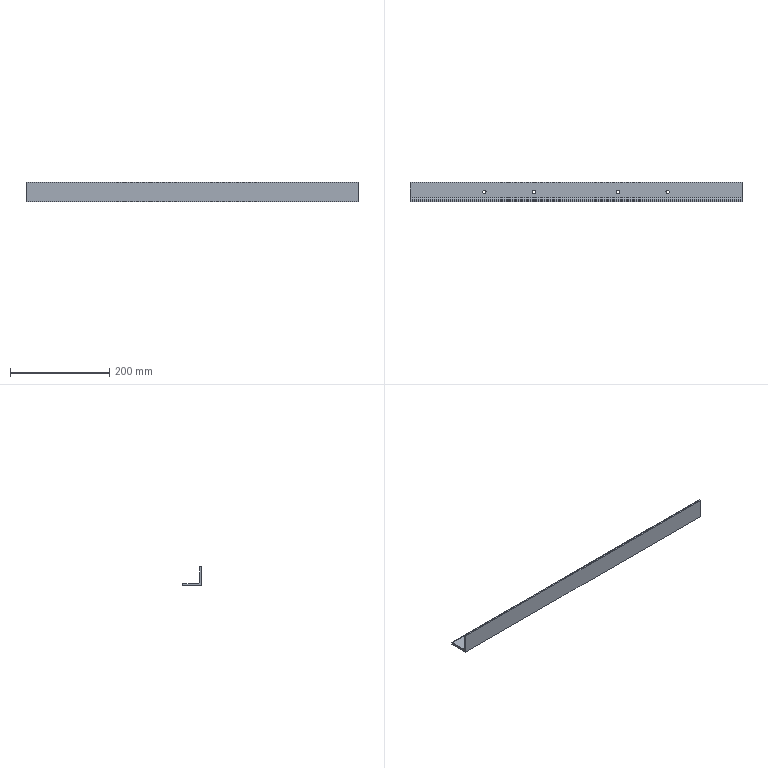Part | SolidWorks | features BaseBody 1 | 1 solid | 19 faces | box 670 x 40 x 40 mm | volume 206182 mm3 | cylinder 11 | plane 8 | commonest cylinder face diameters 6.8 x8 2.667 x2 10 x1
STEP:
#1=CARTESIAN_POINT('',(188.4,20.,4.));
#2=VERTEX_POINT('',#1);
#3=CARTESIAN_POINT('',(181.6,20.,4.));
#4=VERTEX_POINT('',#3);
#5=CARTESIAN_POINT('',(185.,20.,4.));
#6=DIRECTION('',(0.,0.,-1.));
#7=DIRECTION('',(0.,1.,0.));
#8=AXIS2_PLACEMENT_3D('',#5,#6,#7);
#9=CIRCLE('',#8,3.4);
#10=EDGE_CURVE('',#2,#4,#9,.T.);
#11=ORIENTED_EDGE('',*,*,#10,.F.);
#12=CARTESIAN_POINT('',(188.4,20.,0.));
#13=VERTEX_POINT('',#12);
#14=CARTESIAN_POINT('',(188.4,20.,0.));
#15=DIRECTION('',(0.,0.,-1.));
#16=VECTOR('',#15,1000.);
#17=LINE('',#14,#16);
#18=EDGE_CURVE('',#2,#13,#17,.T.);
#19=ORIENTED_EDGE('',*,*,#18,.T.);
#20=CARTESIAN_POINT('',(181.6,20.,0.));
#21=VERTEX_POINT('',#20);
#22=CARTESIAN_POINT('',(185.,20.,0.));
#23=DIRECTION('',(0.,0.,-1.));
#24=DIRECTION('',(-1.,0.,0.));
#25=AXIS2_PLACEMENT_3D('',#22,#23,#24);
#26=CIRCLE('',#25,3.4);
#27=EDGE_CURVE('',#13,#21,#26,.T.);
#28=ORIENTED_EDGE('',*,*,#27,.T.);
#29=CARTESIAN_POINT('',(181.6,20.,0.));
#30=DIRECTION('',(0.,0.,-1.));
#31=VECTOR('',#30,1000.);
#32=LINE('',#29,#31);
#33=EDGE_CURVE('',#4,#21,#32,.T.);
#34=ORIENTED_EDGE('',*,*,#33,.F.);
#35=EDGE_LOOP('',(#11,#19,#28,#34));
#36=FACE_OUTER_BOUND('',#35,.T.);
#37=CARTESIAN_POINT('',(185.,20.,0.));
#38=DIRECTION('',(0.,0.,-1.));
#39=DIRECTION('',(-1.,0.,0.));
#40=AXIS2_PLACEMENT_3D('',#37,#38,#39);
#41=CYLINDRICAL_SURFACE('',#40,3.4);
#42=ADVANCED_FACE('',(#36),#41,.F.);
#43=CARTESIAN_POINT('',(88.4,20.,4.));
#44=VERTEX_POINT('',#43);
#45=CARTESIAN_POINT('',(81.6,20.,4.));
#46=VERTEX_POINT('',#45);
#47=CARTESIAN_POINT('',(85.,20.,4.));
#48=DIRECTION('',(0.,0.,-1.));
#49=DIRECTION('',(0.,1.,0.));
#50=AXIS2_PLACEMENT_3D('',#47,#48,#49);
#51=CIRCLE('',#50,3.4);
#52=EDGE_CURVE('',#44,#46,#51,.T.);
#53=ORIENTED_EDGE('',*,*,#52,.F.);
#54=CARTESIAN_POINT('',(88.4,20.,0.));
#55=VERTEX_POINT('',#54);
#56=CARTESIAN_POINT('',(88.4,20.,0.));
#57=DIRECTION('',(0.,0.,-1.));
#58=VECTOR('',#57,1000.);
#59=LINE('',#56,#58);
#60=EDGE_CURVE('',#44,#55,#59,.T.);
#61=ORIENTED_EDGE('',*,*,#60,.T.);
#62=CARTESIAN_POINT('',(81.6,20.,0.));
#63=VERTEX_POINT('',#62);
#64=CARTESIAN_POINT('',(85.,20.,0.));
#65=DIRECTION('',(0.,0.,-1.));
#66=DIRECTION('',(-1.,0.,0.));
#67=AXIS2_PLACEMENT_3D('',#64,#65,#66);
#68=CIRCLE('',#67,3.4);
#69=EDGE_CURVE('',#55,#63,#68,.T.);
#70=ORIENTED_EDGE('',*,*,#69,.T.);
#71=CARTESIAN_POINT('',(81.6,20.,0.));
#72=DIRECTION('',(0.,0.,-1.));
#73=VECTOR('',#72,1000.);
#74=LINE('',#71,#73);
#75=EDGE_CURVE('',#46,#63,#74,.T.);
#76=ORIENTED_EDGE('',*,*,#75,.F.);
#77=EDGE_LOOP('',(#53,#61,#70,#76));
#78=FACE_OUTER_BOUND('',#77,.T.);
#79=CARTESIAN_POINT('',(85.,20.,0.));
#80=DIRECTION('',(0.,0.,-1.));
#81=DIRECTION('',(-1.,0.,0.));
#82=AXIS2_PLACEMENT_3D('',#79,#80,#81);
#83=CYLINDRICAL_SURFACE('',#82,3.4);
#84=ADVANCED_FACE('',(#78),#83,.F.);
#85=CARTESIAN_POINT('',(-181.6,20.,4.));
#86=VERTEX_POINT('',#85);
#87=CARTESIAN_POINT('',(-188.4,20.,4.));
#88=VERTEX_POINT('',#87);
#89=CARTESIAN_POINT('',(-185.,20.,4.));
#90=DIRECTION('',(0.,0.,-1.));
#91=DIRECTION('',(0.,1.,0.));
#92=AXIS2_PLACEMENT_3D('',#89,#90,#91);
#93=CIRCLE('',#92,3.4);
#94=EDGE_CURVE('',#86,#88,#93,.T.);
#95=ORIENTED_EDGE('',*,*,#94,.F.);
#96=CARTESIAN_POINT('',(-181.6,20.,0.));
#97=VERTEX_POINT('',#96);
#98=CARTESIAN_POINT('',(-181.6,20.,0.));
#99=DIRECTION('',(0.,0.,-1.));
#100=VECTOR('',#99,1000.);
#101=LINE('',#98,#100);
#102=EDGE_CURVE('',#86,#97,#101,.T.);
#103=ORIENTED_EDGE('',*,*,#102,.T.);
#104=CARTESIAN_POINT('',(-188.4,20.,0.));
#105=VERTEX_POINT('',#104);
#106=CARTESIAN_POINT('',(-185.,20.,0.));
#107=DIRECTION('',(0.,0.,-1.));
#108=DIRECTION('',(-1.,0.,0.));
#109=AXIS2_PLACEMENT_3D('',#106,#107,#108);
#110=CIRCLE('',#109,3.4);
#111=EDGE_CURVE('',#97,#105,#110,.T.);
#112=ORIENTED_EDGE('',*,*,#111,.T.);
#113=CARTESIAN_POINT('',(-188.4,20.,0.));
#114=DIRECTION('',(0.,0.,-1.));
#115=VECTOR('',#114,1000.);
#116=LINE('',#113,#115);
#117=EDGE_CURVE('',#88,#105,#116,.T.);
#118=ORIENTED_EDGE('',*,*,#117,.F.);
#119=EDGE_LOOP('',(#95,#103,#112,#118));
#120=FACE_OUTER_BOUND('',#119,.T.);
#121=CARTESIAN_POINT('',(-185.,20.,0.));
#122=DIRECTION('',(0.,0.,-1.));
#123=DIRECTION('',(-1.,0.,0.));
#124=AXIS2_PLACEMENT_3D('',#121,#122,#123);
#125=CYLINDRICAL_SURFACE('',#124,3.4);
#126=ADVANCED_FACE('',(#120),#125,.F.);
#127=CARTESIAN_POINT('',(-81.6,20.,4.));
#128=VERTEX_POINT('',#127);
#129=CARTESIAN_POINT('',(-88.4,20.,4.));
#130=VERTEX_POINT('',#129);
#131=CARTESIAN_POINT('',(-85.,20.,4.));
#132=DIRECTION('',(0.,0.,-1.));
#133=DIRECTION('',(0.,1.,0.));
#134=AXIS2_PLACEMENT_3D('',#131,#132,#133);
#135=CIRCLE('',#134,3.4);
#136=EDGE_CURVE('',#128,#130,#135,.T.);
#137=ORIENTED_EDGE('',*,*,#136,.F.);
#138=CARTESIAN_POINT('',(-81.6,20.,0.));
#139=VERTEX_POINT('',#138);
#140=CARTESIAN_POINT('',(-81.6,20.,0.));
#141=DIRECTION('',(0.,0.,-1.));
#142=VECTOR('',#141,1000.);
#143=LINE('',#140,#142);
#144=EDGE_CURVE('',#128,#139,#143,.T.);
#145=ORIENTED_EDGE('',*,*,#144,.T.);
#146=CARTESIAN_POINT('',(-88.4,20.,0.));
#147=VERTEX_POINT('',#146);
#148=CARTESIAN_POINT('',(-85.,20.,0.));
#149=DIRECTION('',(0.,0.,-1.));
#150=DIRECTION('',(-1.,0.,0.));
#151=AXIS2_PLACEMENT_3D('',#148,#149,#150);
#152=CIRCLE('',#151,3.4);
#153=EDGE_CURVE('',#139,#147,#152,.T.);
#154=ORIENTED_EDGE('',*,*,#153,.T.);
#155=CARTESIAN_POINT('',(-88.4,20.,0.));
#156=DIRECTION('',(0.,0.,-1.));
#157=VECTOR('',#156,1000.);
#158=LINE('',#155,#157);
#159=EDGE_CURVE('',#130,#147,#158,.T.);
#160=ORIENTED_EDGE('',*,*,#159,.F.);
#161=EDGE_LOOP('',(#137,#145,#154,#160));
#162=FACE_OUTER_BOUND('',#161,.T.);
#163=CARTESIAN_POINT('',(-85.,20.,0.));
#164=DIRECTION('',(0.,0.,-1.));
#165=DIRECTION('',(-1.,0.,0.));
#166=AXIS2_PLACEMENT_3D('',#163,#164,#165);
#167=CYLINDRICAL_SURFACE('',#166,3.4);
#168=ADVANCED_FACE('',(#162),#167,.F.);
#169=CARTESIAN_POINT('',(185.,20.,0.));
#170=DIRECTION('',(0.,0.,-1.));
#171=DIRECTION('',(-1.,0.,0.));
#172=AXIS2_PLACEMENT_3D('',#169,#170,#171);
#173=CIRCLE('',#172,3.4);
#174=EDGE_CURVE('',#21,#13,#173,.T.);
#175=ORIENTED_EDGE('',*,*,#174,.F.);
#176=ORIENTED_EDGE('',*,*,#27,.F.);
#177=EDGE_LOOP('',(#175,#176));
#178=FACE_BOUND('',#177,.T.);
#179=CARTESIAN_POINT('',(85.,20.,0.));
#180=DIRECTION('',(0.,0.,-1.));
#181=DIRECTION('',(-1.,0.,0.));
#182=AXIS2_PLACEMENT_3D('',#179,#180,#181);
#183=CIRCLE('',#182,3.4);
#184=EDGE_CURVE('',#63,#55,#183,.T.);
#185=ORIENTED_EDGE('',*,*,#184,.F.);
#186=ORIENTED_EDGE('',*,*,#69,.F.);
#187=EDGE_LOOP('',(#185,#186));
#188=FACE_BOUND('',#187,.T.);
#189=CARTESIAN_POINT('',(-185.,20.,0.));
#190=DIRECTION('',(0.,0.,-1.));
#191=DIRECTION('',(-1.,0.,0.));
#192=AXIS2_PLACEMENT_3D('',#189,#190,#191);
#193=CIRCLE('',#192,3.4);
#194=EDGE_CURVE('',#105,#97,#193,.T.);
#195=ORIENTED_EDGE('',*,*,#194,.F.);
#196=ORIENTED_EDGE('',*,*,#111,.F.);
#197=EDGE_LOOP('',(#195,#196));
#198=FACE_BOUND('',#197,.T.);
#199=CARTESIAN_POINT('',(-85.,20.,0.));
#200=DIRECTION('',(0.,0.,-1.));
#201=DIRECTION('',(-1.,0.,0.));
#202=AXIS2_PLACEMENT_3D('',#199,#200,#201);
#203=CIRCLE('',#202,3.4);
#204=EDGE_CURVE('',#147,#139,#203,.T.);
#205=ORIENTED_EDGE('',*,*,#204,.F.);
#206=ORIENTED_EDGE('',*,*,#153,.F.);
#207=EDGE_LOOP('',(#205,#206));
#208=FACE_BOUND('',#207,.T.);
#209=CARTESIAN_POINT('',(-335.,0.,0.));
#210=VERTEX_POINT('',#209);
#211=CARTESIAN_POINT('',(-335.,40.,0.));
#212=VERTEX_POINT('',#211);
#213=CARTESIAN_POINT('',(-335.,40.,0.));
#214=DIRECTION('',(0.,1.,0.));
#215=VECTOR('',#214,1000.);
#216=LINE('',#213,#215);
#217=EDGE_CURVE('',#210,#212,#216,.T.);
#218=ORIENTED_EDGE('',*,*,#217,.T.);
#219=CARTESIAN_POINT('',(335.,40.,0.));
#220=VERTEX_POINT('',#219);
#221=CARTESIAN_POINT('',(335.,40.,0.));
#222=DIRECTION('',(-1.,0.,0.));
#223=VECTOR('',#222,1000.);
#224=LINE('',#221,#223);
#225=EDGE_CURVE('',#220,#212,#224,.T.);
#226=ORIENTED_EDGE('',*,*,#225,.F.);
#227=CARTESIAN_POINT('',(335.,0.,0.));
#228=VERTEX_POINT('',#227);
#229=CARTESIAN_POINT('',(335.,40.,0.));
#230=DIRECTION('',(0.,1.,0.));
#231=VECTOR('',#230,1000.);
#232=LINE('',#229,#231);
#233=EDGE_CURVE('',#228,#220,#232,.T.);
#234=ORIENTED_EDGE('',*,*,#233,.F.);
#235=CARTESIAN_POINT('',(335.,0.,0.));
#236=DIRECTION('',(-1.,0.,0.));
#237=VECTOR('',#236,1000.);
#238=LINE('',#235,#237);
#239=EDGE_CURVE('',#228,#210,#238,.T.);
#240=ORIENTED_EDGE('',*,*,#239,.T.);
#241=EDGE_LOOP('',(#218,#226,#234,#240));
#242=FACE_OUTER_BOUND('',#241,.T.);
#243=CARTESIAN_POINT('',(335.,40.,0.));
#244=DIRECTION('',(0.,0.,1.));
#245=DIRECTION('',(1.,0.,0.));
#246=AXIS2_PLACEMENT_3D('',#243,#244,#245);
#247=PLANE('',#246);
#248=ADVANCED_FACE('',(#178,#188,#198,#208,#242),#247,.F.);
#249=CARTESIAN_POINT('',(-335.,40.,2.667));
#250=VERTEX_POINT('',#249);
#251=CARTESIAN_POINT('',(-335.,40.,0.));
#252=DIRECTION('',(0.,0.,1.));
#253=VECTOR('',#252,1000.);
#254=LINE('',#251,#253);
#255=EDGE_CURVE('',#212,#250,#254,.T.);
#256=ORIENTED_EDGE('',*,*,#255,.T.);
#257=CARTESIAN_POINT('',(335.,40.,2.667));
#258=VERTEX_POINT('',#257);
#259=CARTESIAN_POINT('',(335.,40.,2.667));
#260=DIRECTION('',(-1.,0.,0.));
#261=VECTOR('',#260,1000.);
#262=LINE('',#259,#261);
#263=EDGE_CURVE('',#258,#250,#262,.T.);
#264=ORIENTED_EDGE('',*,*,#263,.F.);
#265=CARTESIAN_POINT('',(335.,40.,0.));
#266=DIRECTION('',(0.,0.,1.));
#267=VECTOR('',#266,1000.);
#268=LINE('',#265,#267);
#269=EDGE_CURVE('',#220,#258,#268,.T.);
#270=ORIENTED_EDGE('',*,*,#269,.F.);
#271=ORIENTED_EDGE('',*,*,#225,.T.);
#272=EDGE_LOOP('',(#256,#264,#270,#271));
#273=FACE_OUTER_BOUND('',#272,.T.);
#274=CARTESIAN_POINT('',(335.,40.,0.));
#275=DIRECTION('',(0.,-1.,0.));
#276=DIRECTION('',(0.,0.,-1.));
#277=AXIS2_PLACEMENT_3D('',#274,#275,#276);
#278=PLANE('',#277);
#279=ADVANCED_FACE('',(#273),#278,.F.);
#280=CARTESIAN_POINT('',(-335.,38.667,4.));
#281=VERTEX_POINT('',#280);
#282=CARTESIAN_POINT('',(-335.,38.667,2.667));
#283=DIRECTION('',(1.,0.,0.));
#284=DIRECTION('',(0.,0.,-1.));
#285=AXIS2_PLACEMENT_3D('',#282,#283,#284);
#286=CIRCLE('',#285,1.333);
#287=EDGE_CURVE('',#250,#281,#286,.T.);
#288=ORIENTED_EDGE('',*,*,#287,.T.);
#289=CARTESIAN_POINT('',(335.,38.667,4.));
#290=VERTEX_POINT('',#289);
#291=CARTESIAN_POINT('',(335.,38.667,4.));
#292=DIRECTION('',(-1.,0.,0.));
#293=VECTOR('',#292,1000.);
#294=LINE('',#291,#293);
#295=EDGE_CURVE('',#290,#281,#294,.T.);
#296=ORIENTED_EDGE('',*,*,#295,.F.);
#297=CARTESIAN_POINT('',(335.,38.667,2.667));
#298=DIRECTION('',(1.,0.,0.));
#299=DIRECTION('',(0.,0.,-1.));
#300=AXIS2_PLACEMENT_3D('',#297,#298,#299);
#301=CIRCLE('',#300,1.333);
#302=EDGE_CURVE('',#258,#290,#301,.T.);
#303=ORIENTED_EDGE('',*,*,#302,.F.);
#304=ORIENTED_EDGE('',*,*,#263,.T.);
#305=EDGE_LOOP('',(#288,#296,#303,#304));
#306=FACE_OUTER_BOUND('',#305,.T.);
#307=CARTESIAN_POINT('',(335.,38.667,2.667));
#308=DIRECTION('',(-1.,0.,0.));
#309=DIRECTION('',(0.,0.,1.));
#310=AXIS2_PLACEMENT_3D('',#307,#308,#309);
#311=CYLINDRICAL_SURFACE('',#310,1.333);
#312=ADVANCED_FACE('',(#306),#311,.T.);
#313=CARTESIAN_POINT('',(185.,20.,4.));
#314=DIRECTION('',(0.,0.,-1.));
#315=DIRECTION('',(0.,1.,0.));
#316=AXIS2_PLACEMENT_3D('',#313,#314,#315);
#317=CIRCLE('',#316,3.4);
#318=EDGE_CURVE('',#4,#2,#317,.T.);
#319=ORIENTED_EDGE('',*,*,#318,.T.);
#320=ORIENTED_EDGE('',*,*,#10,.T.);
#321=EDGE_LOOP('',(#319,#320));
#322=FACE_BOUND('',#321,.T.);
#323=CARTESIAN_POINT('',(85.,20.,4.));
#324=DIRECTION('',(0.,0.,-1.));
#325=DIRECTION('',(0.,1.,0.));
#326=AXIS2_PLACEMENT_3D('',#323,#324,#325);
#327=CIRCLE('',#326,3.4);
#328=EDGE_CURVE('',#46,#44,#327,.T.);
#329=ORIENTED_EDGE('',*,*,#328,.T.);
#330=ORIENTED_EDGE('',*,*,#52,.T.);
#331=EDGE_LOOP('',(#329,#330));
#332=FACE_BOUND('',#331,.T.);
#333=CARTESIAN_POINT('',(-185.,20.,4.));
#334=DIRECTION('',(0.,0.,-1.));
#335=DIRECTION('',(0.,1.,0.));
#336=AXIS2_PLACEMENT_3D('',#333,#334,#335);
#337=CIRCLE('',#336,3.4);
#338=EDGE_CURVE('',#88,#86,#337,.T.);
#339=ORIENTED_EDGE('',*,*,#338,.T.);
#340=ORIENTED_EDGE('',*,*,#94,.T.);
#341=EDGE_LOOP('',(#339,#340));
#342=FACE_BOUND('',#341,.T.);
#343=CARTESIAN_POINT('',(-85.,20.,4.));
#344=DIRECTION('',(0.,0.,-1.));
#345=DIRECTION('',(0.,1.,0.));
#346=AXIS2_PLACEMENT_3D('',#343,#344,#345);
#347=CIRCLE('',#346,3.4);
#348=EDGE_CURVE('',#130,#128,#347,.T.);
#349=ORIENTED_EDGE('',*,*,#348,.T.);
#350=ORIENTED_EDGE('',*,*,#136,.T.);
#351=EDGE_LOOP('',(#349,#350));
#352=FACE_BOUND('',#351,.T.);
#353=CARTESIAN_POINT('',(-335.,9.,4.));
#354=VERTEX_POINT('',#353);
#355=CARTESIAN_POINT('',(-335.,9.,4.));
#356=DIRECTION('',(0.,-1.,0.));
#357=VECTOR('',#356,1000.);
#358=LINE('',#355,#357);
#359=EDGE_CURVE('',#281,#354,#358,.T.);
#360=ORIENTED_EDGE('',*,*,#359,.T.);
#361=CARTESIAN_POINT('',(335.,9.,4.));
#362=VERTEX_POINT('',#361);
#363=CARTESIAN_POINT('',(335.,9.,4.));
#364=DIRECTION('',(-1.,0.,0.));
#365=VECTOR('',#364,1000.);
#366=LINE('',#363,#365);
#367=EDGE_CURVE('',#362,#354,#366,.T.);
#368=ORIENTED_EDGE('',*,*,#367,.F.);
#369=CARTESIAN_POINT('',(335.,9.,4.));
#370=DIRECTION('',(0.,-1.,0.));
#371=VECTOR('',#370,1000.);
#372=LINE('',#369,#371);
#373=EDGE_CURVE('',#290,#362,#372,.T.);
#374=ORIENTED_EDGE('',*,*,#373,.F.);
#375=ORIENTED_EDGE('',*,*,#295,.T.);
#376=EDGE_LOOP('',(#360,#368,#374,#375));
#377=FACE_OUTER_BOUND('',#376,.T.);
#378=CARTESIAN_POINT('',(335.,9.,4.));
#379=DIRECTION('',(0.,0.,-1.));
#380=DIRECTION('',(0.,1.,0.));
#381=AXIS2_PLACEMENT_3D('',#378,#379,#380);
#382=PLANE('',#381);
#383=ADVANCED_FACE('',(#322,#332,#342,#352,#377),#382,.F.);
#384=CARTESIAN_POINT('',(-335.,4.,9.));
#385=VERTEX_POINT('',#384);
#386=CARTESIAN_POINT('',(-335.,9.,9.));
#387=DIRECTION('',(-1.,0.,0.));
#388=DIRECTION('',(0.,0.,1.));
#389=AXIS2_PLACEMENT_3D('',#386,#387,#388);
#390=CIRCLE('',#389,5.);
#391=EDGE_CURVE('',#354,#385,#390,.T.);
#392=ORIENTED_EDGE('',*,*,#391,.T.);
#393=CARTESIAN_POINT('',(335.,4.,9.));
#394=VERTEX_POINT('',#393);
#395=CARTESIAN_POINT('',(335.,4.,9.));
#396=DIRECTION('',(-1.,0.,0.));
#397=VECTOR('',#396,1000.);
#398=LINE('',#395,#397);
#399=EDGE_CURVE('',#394,#385,#398,.T.);
#400=ORIENTED_EDGE('',*,*,#399,.F.);
#401=CARTESIAN_POINT('',(335.,9.,9.));
#402=DIRECTION('',(-1.,0.,0.));
#403=DIRECTION('',(0.,0.,1.));
#404=AXIS2_PLACEMENT_3D('',#401,#402,#403);
#405=CIRCLE('',#404,5.);
#406=EDGE_CURVE('',#362,#394,#405,.T.);
#407=ORIENTED_EDGE('',*,*,#406,.F.);
#408=ORIENTED_EDGE('',*,*,#367,.T.);
#409=EDGE_LOOP('',(#392,#400,#407,#408));
#410=FACE_OUTER_BOUND('',#409,.T.);
#411=CARTESIAN_POINT('',(335.,9.,9.));
#412=DIRECTION('',(-1.,0.,0.));
#413=DIRECTION('',(0.,0.,1.));
#414=AXIS2_PLACEMENT_3D('',#411,#412,#413);
#415=CYLINDRICAL_SURFACE('',#414,5.);
#416=ADVANCED_FACE('',(#410),#415,.F.);
#417=CARTESIAN_POINT('',(-335.,4.,38.667));
#418=VERTEX_POINT('',#417);
#419=CARTESIAN_POINT('',(-335.,4.,38.667));
#420=DIRECTION('',(0.,0.,1.));
#421=VECTOR('',#420,1000.);
#422=LINE('',#419,#421);
#423=EDGE_CURVE('',#385,#418,#422,.T.);
#424=ORIENTED_EDGE('',*,*,#423,.T.);
#425=CARTESIAN_POINT('',(335.,4.,38.667));
#426=VERTEX_POINT('',#425);
#427=CARTESIAN_POINT('',(335.,4.,38.667));
#428=DIRECTION('',(-1.,0.,0.));
#429=VECTOR('',#428,1000.);
#430=LINE('',#427,#429);
#431=EDGE_CURVE('',#426,#418,#430,.T.);
#432=ORIENTED_EDGE('',*,*,#431,.F.);
#433=CARTESIAN_POINT('',(335.,4.,38.667));
#434=DIRECTION('',(0.,0.,1.));
#435=VECTOR('',#434,1000.);
#436=LINE('',#433,#435);
#437=EDGE_CURVE('',#394,#426,#436,.T.);
#438=ORIENTED_EDGE('',*,*,#437,.F.);
#439=ORIENTED_EDGE('',*,*,#399,.T.);
#440=EDGE_LOOP('',(#424,#432,#438,#439));
#441=FACE_OUTER_BOUND('',#440,.T.);
#442=CARTESIAN_POINT('',(335.,4.,38.667));
#443=DIRECTION('',(0.,-1.,0.));
#444=DIRECTION('',(0.,0.,-1.));
#445=AXIS2_PLACEMENT_3D('',#442,#443,#444);
#446=PLANE('',#445);
#447=ADVANCED_FACE('',(#441),#446,.F.);
#448=CARTESIAN_POINT('',(-335.,2.667,40.));
#449=VERTEX_POINT('',#448);
#450=CARTESIAN_POINT('',(-335.,2.667,38.667));
#451=DIRECTION('',(1.,0.,0.));
#452=DIRECTION('',(0.,0.,1.));
#453=AXIS2_PLACEMENT_3D('',#450,#451,#452);
#454=CIRCLE('',#453,1.333);
#455=EDGE_CURVE('',#418,#449,#454,.T.);
#456=ORIENTED_EDGE('',*,*,#455,.T.);
#457=CARTESIAN_POINT('',(335.,2.667,40.));
#458=VERTEX_POINT('',#457);
#459=CARTESIAN_POINT('',(335.,2.667,40.));
#460=DIRECTION('',(-1.,0.,0.));
#461=VECTOR('',#460,1000.);
#462=LINE('',#459,#461);
#463=EDGE_CURVE('',#458,#449,#462,.T.);
#464=ORIENTED_EDGE('',*,*,#463,.F.);
#465=CARTESIAN_POINT('',(335.,2.667,38.667));
#466=DIRECTION('',(1.,0.,0.));
#467=DIRECTION('',(0.,0.,1.));
#468=AXIS2_PLACEMENT_3D('',#465,#466,#467);
#469=CIRCLE('',#468,1.333);
#470=EDGE_CURVE('',#426,#458,#469,.T.);
#471=ORIENTED_EDGE('',*,*,#470,.F.);
#472=ORIENTED_EDGE('',*,*,#431,.T.);
#473=EDGE_LOOP('',(#456,#464,#471,#472));
#474=FACE_OUTER_BOUND('',#473,.T.);
#475=CARTESIAN_POINT('',(335.,2.667,38.667));
#476=DIRECTION('',(-1.,0.,0.));
#477=DIRECTION('',(0.,0.,1.));
#478=AXIS2_PLACEMENT_3D('',#475,#476,#477);
#479=CYLINDRICAL_SURFACE('',#478,1.333);
#480=ADVANCED_FACE('',(#474),#479,.T.);
#481=CARTESIAN_POINT('',(-335.,0.,40.));
#482=VERTEX_POINT('',#481);
#483=CARTESIAN_POINT('',(-335.,0.,40.));
#484=DIRECTION('',(0.,-1.,0.));
#485=VECTOR('',#484,1000.);
#486=LINE('',#483,#485);
#487=EDGE_CURVE('',#449,#482,#486,.T.);
#488=ORIENTED_EDGE('',*,*,#487,.T.);
#489=CARTESIAN_POINT('',(335.,0.,40.));
#490=VERTEX_POINT('',#489);
#491=CARTESIAN_POINT('',(335.,0.,40.));
#492=DIRECTION('',(-1.,0.,0.));
#493=VECTOR('',#492,1000.);
#494=LINE('',#491,#493);
#495=EDGE_CURVE('',#490,#482,#494,.T.);
#496=ORIENTED_EDGE('',*,*,#495,.F.);
#497=CARTESIAN_POINT('',(335.,0.,40.));
#498=DIRECTION('',(0.,-1.,0.));
#499=VECTOR('',#498,1000.);
#500=LINE('',#497,#499);
#501=EDGE_CURVE('',#458,#490,#500,.T.);
#502=ORIENTED_EDGE('',*,*,#501,.F.);
#503=ORIENTED_EDGE('',*,*,#463,.T.);
#504=EDGE_LOOP('',(#488,#496,#502,#503));
#505=FACE_OUTER_BOUND('',#504,.T.);
#506=CARTESIAN_POINT('',(335.,0.,40.));
#507=DIRECTION('',(0.,0.,-1.));
#508=DIRECTION('',(-1.,0.,0.));
#509=AXIS2_PLACEMENT_3D('',#506,#507,#508);
#510=PLANE('',#509);
#511=ADVANCED_FACE('',(#505),#510,.F.);
#512=CARTESIAN_POINT('',(-335.,0.,0.));
#513=DIRECTION('',(0.,0.,-1.));
#514=VECTOR('',#513,1000.);
#515=LINE('',#512,#514);
#516=EDGE_CURVE('',#482,#210,#515,.T.);
#517=ORIENTED_EDGE('',*,*,#516,.T.);
#518=ORIENTED_EDGE('',*,*,#239,.F.);
#519=CARTESIAN_POINT('',(335.,0.,0.));
#520=DIRECTION('',(0.,0.,-1.));
#521=VECTOR('',#520,1000.);
#522=LINE('',#519,#521);
#523=EDGE_CURVE('',#490,#228,#522,.T.);
#524=ORIENTED_EDGE('',*,*,#523,.F.);
#525=ORIENTED_EDGE('',*,*,#495,.T.);
#526=EDGE_LOOP('',(#517,#518,#524,#525));
#527=FACE_OUTER_BOUND('',#526,.T.);
#528=CARTESIAN_POINT('',(335.,0.,0.));
#529=DIRECTION('',(0.,1.,0.));
#530=DIRECTION('',(0.,0.,1.));
#531=AXIS2_PLACEMENT_3D('',#528,#529,#530);
#532=PLANE('',#531);
#533=ADVANCED_FACE('',(#527),#532,.F.);
#534=ORIENTED_EDGE('',*,*,#233,.T.);
#535=ORIENTED_EDGE('',*,*,#269,.T.);
#536=ORIENTED_EDGE('',*,*,#302,.T.);
#537=ORIENTED_EDGE('',*,*,#373,.T.);
#538=ORIENTED_EDGE('',*,*,#406,.T.);
#539=ORIENTED_EDGE('',*,*,#437,.T.);
#540=ORIENTED_EDGE('',*,*,#470,.T.);
#541=ORIENTED_EDGE('',*,*,#501,.T.);
#542=ORIENTED_EDGE('',*,*,#523,.T.);
#543=EDGE_LOOP('',(#534,#535,#536,#537,#538,#539,#540,#541,#542));
#544=FACE_OUTER_BOUND('',#543,.T.);
#545=CARTESIAN_POINT('',(335.,2.667,38.667));
#546=DIRECTION('',(-1.,0.,0.));
#547=DIRECTION('',(0.,0.,1.));
#548=AXIS2_PLACEMENT_3D('',#545,#546,#547);
#549=PLANE('',#548);
#550=ADVANCED_FACE('',(#544),#549,.F.);
#551=ORIENTED_EDGE('',*,*,#217,.F.);
#552=ORIENTED_EDGE('',*,*,#516,.F.);
#553=ORIENTED_EDGE('',*,*,#487,.F.);
#554=ORIENTED_EDGE('',*,*,#455,.F.);
#555=ORIENTED_EDGE('',*,*,#423,.F.);
#556=ORIENTED_EDGE('',*,*,#391,.F.);
#557=ORIENTED_EDGE('',*,*,#359,.F.);
#558=ORIENTED_EDGE('',*,*,#287,.F.);
#559=ORIENTED_EDGE('',*,*,#255,.F.);
#560=EDGE_LOOP('',(#551,#552,#553,#554,#555,#556,#557,#558,#559));
#561=FACE_OUTER_BOUND('',#560,.T.);
#562=CARTESIAN_POINT('',(-335.,2.667,38.667));
#563=DIRECTION('',(-1.,0.,0.));
#564=DIRECTION('',(0.,0.,1.));
#565=AXIS2_PLACEMENT_3D('',#562,#563,#564);
#566=PLANE('',#565);
#567=ADVANCED_FACE('',(#561),#566,.T.);
#568=ORIENTED_EDGE('',*,*,#144,.F.);
#569=ORIENTED_EDGE('',*,*,#348,.F.);
#570=ORIENTED_EDGE('',*,*,#159,.T.);
#571=ORIENTED_EDGE('',*,*,#204,.T.);
#572=EDGE_LOOP('',(#568,#569,#570,#571));
#573=FACE_OUTER_BOUND('',#572,.T.);
#574=CARTESIAN_POINT('',(-85.,20.,0.));
#575=DIRECTION('',(0.,0.,-1.));
#576=DIRECTION('',(-1.,0.,0.));
#577=AXIS2_PLACEMENT_3D('',#574,#575,#576);
#578=CYLINDRICAL_SURFACE('',#577,3.4);
#579=ADVANCED_FACE('',(#573),#578,.F.);
#580=ORIENTED_EDGE('',*,*,#102,.F.);
#581=ORIENTED_EDGE('',*,*,#338,.F.);
#582=ORIENTED_EDGE('',*,*,#117,.T.);
#583=ORIENTED_EDGE('',*,*,#194,.T.);
#584=EDGE_LOOP('',(#580,#581,#582,#583));
#585=FACE_OUTER_BOUND('',#584,.T.);
#586=CARTESIAN_POINT('',(-185.,20.,0.));
#587=DIRECTION('',(0.,0.,-1.));
#588=DIRECTION('',(-1.,0.,0.));
#589=AXIS2_PLACEMENT_3D('',#586,#587,#588);
#590=CYLINDRICAL_SURFACE('',#589,3.4);
#591=ADVANCED_FACE('',(#585),#590,.F.);
#592=ORIENTED_EDGE('',*,*,#60,.F.);
#593=ORIENTED_EDGE('',*,*,#328,.F.);
#594=ORIENTED_EDGE('',*,*,#75,.T.);
#595=ORIENTED_EDGE('',*,*,#184,.T.);
#596=EDGE_LOOP('',(#592,#593,#594,#595));
#597=FACE_OUTER_BOUND('',#596,.T.);
#598=CARTESIAN_POINT('',(85.,20.,0.));
#599=DIRECTION('',(0.,0.,-1.));
#600=DIRECTION('',(-1.,0.,0.));
#601=AXIS2_PLACEMENT_3D('',#598,#599,#600);
#602=CYLINDRICAL_SURFACE('',#601,3.4);
#603=ADVANCED_FACE('',(#597),#602,.F.);
#604=ORIENTED_EDGE('',*,*,#18,.F.);
#605=ORIENTED_EDGE('',*,*,#318,.F.);
#606=ORIENTED_EDGE('',*,*,#33,.T.);
#607=ORIENTED_EDGE('',*,*,#174,.T.);
#608=EDGE_LOOP('',(#604,#605,#606,#607));
#609=FACE_OUTER_BOUND('',#608,.T.);
#610=CARTESIAN_POINT('',(185.,20.,0.));
#611=DIRECTION('',(0.,0.,-1.));
#612=DIRECTION('',(-1.,0.,0.));
#613=AXIS2_PLACEMENT_3D('',#610,#611,#612);
#614=CYLINDRICAL_SURFACE('',#613,3.4);
#615=ADVANCED_FACE('',(#609),#614,.F.);
#616=CLOSED_SHELL('',(#42,#84,#126,#168,#248,#279,#312,#383,#416,#447,#480,#511,#533,#550,#567,#579,#591,#603,#615));
#617=MANIFOLD_SOLID_BREP('',#616);
#618=CARTESIAN_POINT('',(0.,0.,0.));
#619=DIRECTION('',(0.,0.,1.));
#620=DIRECTION('',(1.,0.,0.));
#621=AXIS2_PLACEMENT_3D('',#618,#619,#620);
#622=(LENGTH_UNIT()NAMED_UNIT(*)SI_UNIT(.MILLI.,.METRE.));
#623=UNCERTAINTY_MEASURE_WITH_UNIT(LENGTH_MEASURE(0.00001),#622,'','');
#624=(NAMED_UNIT(*)PLANE_ANGLE_UNIT()SI_UNIT($,.RADIAN.));
#625=(NAMED_UNIT(*)SI_UNIT($,.STERADIAN.)SOLID_ANGLE_UNIT());
#626=(GEOMETRIC_REPRESENTATION_CONTEXT(3)GLOBAL_UNCERTAINTY_ASSIGNED_CONTEXT((#623))GLOBAL_UNIT_ASSIGNED_CONTEXT((#622,#624,#625))REPRESENTATION_CONTEXT('',''));
#627=ADVANCED_BREP_SHAPE_REPRESENTATION('',(#617,#621),#626);